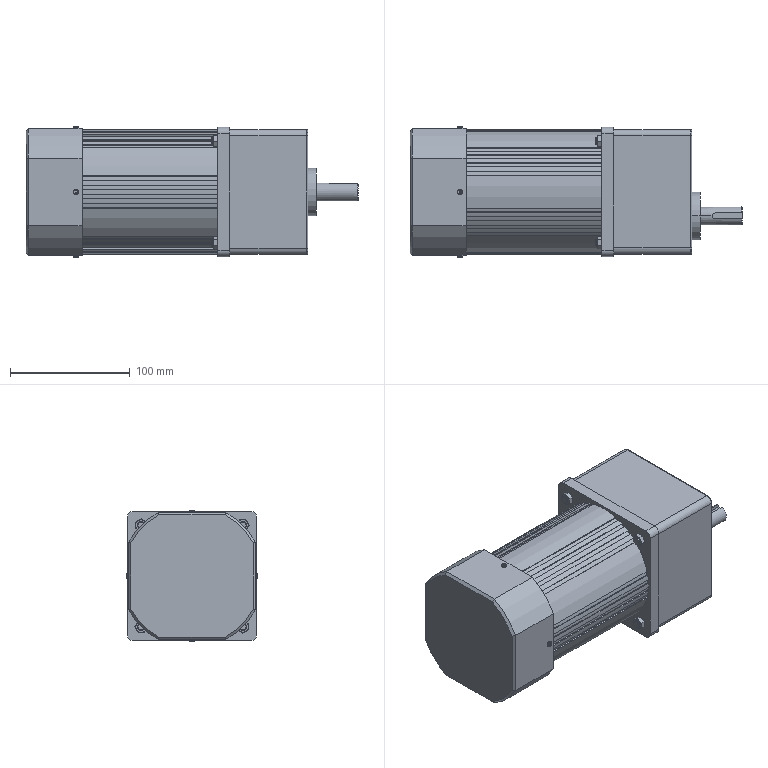Part | SolidWorks | features ICE 13, Fillet 4, Chamfer 3, CirPattern 3, Revolution 2, Extrusion 1, LibraryFeature 1, MoveFace 1 | 2 solids | 331 faces | box 277 x 108.652 x 108.652 mm | volume 2249960 mm3 | plane 164 | cylinder 104 | cone 41 | torus 22 | commonest cylinder face diameters 104 x25 102 x24 4.42 x8 6 x8 9 x8 9.2 x8